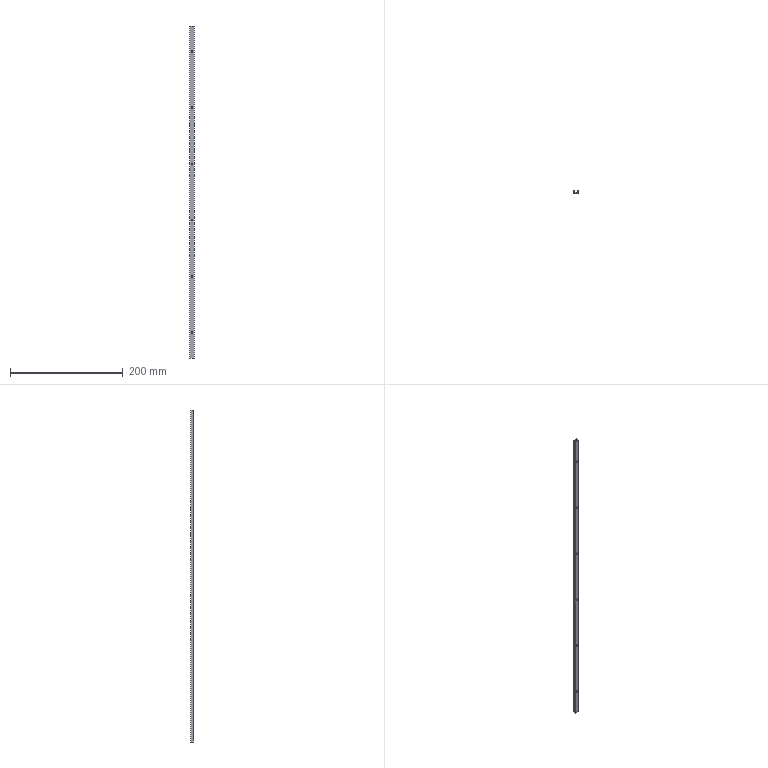Part | STEP file | 1 solid | 30 faces | box 8 x 5 x 590 mm | volume 11867 mm3 | plane 18 | cylinder 12 | commonest cylinder face diameters 3 x12